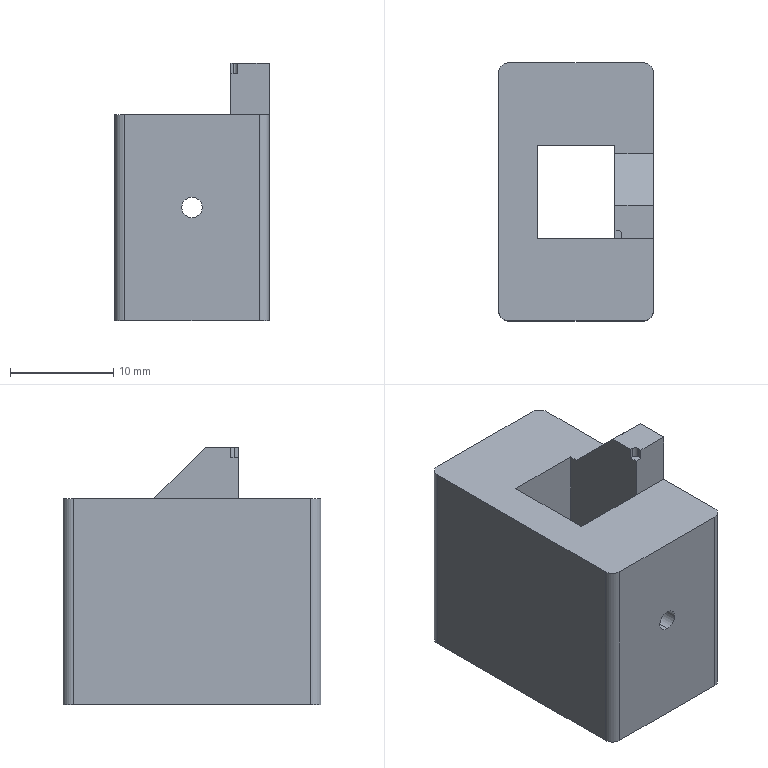Part | STEP file | 03-08 left pre-press cutter plate | 1 solid | 38 faces | box 15 x 25 x 25 mm | volume 5712 mm3 | plane 19 | cylinder 17 | cone 2 | commonest cylinder face diameters 2 x6 3.1 x4 7 x4 4.2 x2 0.7 x1
STEP:
#1=CARTESIAN_POINT('',(0.,-8.5,10.));
#2=VERTEX_POINT('',#1);
#3=CARTESIAN_POINT('',(0.,-8.5,12.));
#4=VERTEX_POINT('',#3);
#5=CARTESIAN_POINT('',(0.,-8.5,11.));
#6=DIRECTION('',(0.,1.,0.));
#7=DIRECTION('',(0.,0.,1.));
#8=AXIS2_PLACEMENT_3D('',#5,#6,#7);
#9=CIRCLE('',#8,1.);
#10=EDGE_CURVE('',#2,#4,#9,.T.);
#11=ORIENTED_EDGE('',*,*,#10,.T.);
#12=CARTESIAN_POINT('',(0.,-12.5,12.));
#13=VERTEX_POINT('',#12);
#14=CARTESIAN_POINT('',(0.,-2.5,12.));
#15=DIRECTION('',(0.,-1.,0.));
#16=VECTOR('',#15,1000.);
#17=LINE('',#14,#16);
#18=EDGE_CURVE('',#4,#13,#17,.T.);
#19=ORIENTED_EDGE('',*,*,#18,.T.);
#20=CARTESIAN_POINT('',(0.,-12.5,10.));
#21=VERTEX_POINT('',#20);
#22=CARTESIAN_POINT('',(0.,-12.5,11.));
#23=DIRECTION('',(0.,-1.,0.));
#24=DIRECTION('',(0.,0.,-1.));
#25=AXIS2_PLACEMENT_3D('',#22,#23,#24);
#26=CIRCLE('',#25,1.);
#27=EDGE_CURVE('',#13,#21,#26,.T.);
#28=ORIENTED_EDGE('',*,*,#27,.T.);
#29=CARTESIAN_POINT('',(0.,-2.5,10.));
#30=DIRECTION('',(0.,-1.,0.));
#31=VECTOR('',#30,1000.);
#32=LINE('',#29,#31);
#33=EDGE_CURVE('',#2,#21,#32,.T.);
#34=ORIENTED_EDGE('',*,*,#33,.F.);
#35=EDGE_LOOP('',(#11,#19,#28,#34));
#36=FACE_OUTER_BOUND('',#35,.T.);
#37=CARTESIAN_POINT('',(0.,-2.5,11.));
#38=DIRECTION('',(0.,-1.,0.));
#39=DIRECTION('',(0.,0.,-1.));
#40=AXIS2_PLACEMENT_3D('',#37,#38,#39);
#41=CYLINDRICAL_SURFACE('',#40,1.);
#42=ADVANCED_FACE('',(#36),#41,.F.);
#43=CARTESIAN_POINT('',(3.5,-8.5,5.));
#44=VERTEX_POINT('',#43);
#45=CARTESIAN_POINT('',(-3.5,-8.5,5.));
#46=VERTEX_POINT('',#45);
#47=CARTESIAN_POINT('',(0.,-8.5,5.));
#48=DIRECTION('',(0.,0.,-1.));
#49=DIRECTION('',(-1.,0.,0.));
#50=AXIS2_PLACEMENT_3D('',#47,#48,#49);
#51=CIRCLE('',#50,3.5);
#52=EDGE_CURVE('',#44,#46,#51,.T.);
#53=ORIENTED_EDGE('',*,*,#52,.F.);
#54=CARTESIAN_POINT('',(3.5,-8.5,0.));
#55=VERTEX_POINT('',#54);
#56=CARTESIAN_POINT('',(3.5,-8.5,5.));
#57=DIRECTION('',(0.,0.,-1.));
#58=VECTOR('',#57,1000.);
#59=LINE('',#56,#58);
#60=EDGE_CURVE('',#44,#55,#59,.T.);
#61=ORIENTED_EDGE('',*,*,#60,.T.);
#62=CARTESIAN_POINT('',(-3.5,-8.5,0.));
#63=VERTEX_POINT('',#62);
#64=CARTESIAN_POINT('',(0.,-8.5,0.));
#65=DIRECTION('',(0.,0.,-1.));
#66=DIRECTION('',(-1.,0.,0.));
#67=AXIS2_PLACEMENT_3D('',#64,#65,#66);
#68=CIRCLE('',#67,3.5);
#69=EDGE_CURVE('',#55,#63,#68,.T.);
#70=ORIENTED_EDGE('',*,*,#69,.T.);
#71=CARTESIAN_POINT('',(-3.5,-8.5,5.));
#72=DIRECTION('',(0.,0.,-1.));
#73=VECTOR('',#72,1000.);
#74=LINE('',#71,#73);
#75=EDGE_CURVE('',#46,#63,#74,.T.);
#76=ORIENTED_EDGE('',*,*,#75,.F.);
#77=EDGE_LOOP('',(#53,#61,#70,#76));
#78=FACE_OUTER_BOUND('',#77,.T.);
#79=CARTESIAN_POINT('',(0.,-8.5,5.));
#80=DIRECTION('',(0.,0.,-1.));
#81=DIRECTION('',(-1.,0.,0.));
#82=AXIS2_PLACEMENT_3D('',#79,#80,#81);
#83=CYLINDRICAL_SURFACE('',#82,3.5);
#84=ADVANCED_FACE('',(#78),#83,.F.);
#85=CARTESIAN_POINT('',(3.5,8.5,5.));
#86=VERTEX_POINT('',#85);
#87=CARTESIAN_POINT('',(-3.5,8.5,5.));
#88=VERTEX_POINT('',#87);
#89=CARTESIAN_POINT('',(0.,8.5,5.));
#90=DIRECTION('',(0.,0.,-1.));
#91=DIRECTION('',(-1.,0.,0.));
#92=AXIS2_PLACEMENT_3D('',#89,#90,#91);
#93=CIRCLE('',#92,3.5);
#94=EDGE_CURVE('',#86,#88,#93,.T.);
#95=ORIENTED_EDGE('',*,*,#94,.F.);
#96=CARTESIAN_POINT('',(3.5,8.5,0.));
#97=VERTEX_POINT('',#96);
#98=CARTESIAN_POINT('',(3.5,8.5,5.));
#99=DIRECTION('',(0.,0.,-1.));
#100=VECTOR('',#99,1000.);
#101=LINE('',#98,#100);
#102=EDGE_CURVE('',#86,#97,#101,.T.);
#103=ORIENTED_EDGE('',*,*,#102,.T.);
#104=CARTESIAN_POINT('',(-3.5,8.5,0.));
#105=VERTEX_POINT('',#104);
#106=CARTESIAN_POINT('',(0.,8.5,0.));
#107=DIRECTION('',(0.,0.,-1.));
#108=DIRECTION('',(-1.,0.,0.));
#109=AXIS2_PLACEMENT_3D('',#106,#107,#108);
#110=CIRCLE('',#109,3.5);
#111=EDGE_CURVE('',#97,#105,#110,.T.);
#112=ORIENTED_EDGE('',*,*,#111,.T.);
#113=CARTESIAN_POINT('',(-3.5,8.5,5.));
#114=DIRECTION('',(0.,0.,-1.));
#115=VECTOR('',#114,1000.);
#116=LINE('',#113,#115);
#117=EDGE_CURVE('',#88,#105,#116,.T.);
#118=ORIENTED_EDGE('',*,*,#117,.F.);
#119=EDGE_LOOP('',(#95,#103,#112,#118));
#120=FACE_OUTER_BOUND('',#119,.T.);
#121=CARTESIAN_POINT('',(0.,8.5,5.));
#122=DIRECTION('',(0.,0.,-1.));
#123=DIRECTION('',(-1.,0.,0.));
#124=AXIS2_PLACEMENT_3D('',#121,#122,#123);
#125=CYLINDRICAL_SURFACE('',#124,3.5);
#126=ADVANCED_FACE('',(#120),#125,.F.);
#127=CARTESIAN_POINT('',(0.,7.5,8.9));
#128=VERTEX_POINT('',#127);
#129=CARTESIAN_POINT('',(0.,7.5,13.1));
#130=VERTEX_POINT('',#129);
#131=CARTESIAN_POINT('',(0.,7.5,11.));
#132=DIRECTION('',(0.,1.,0.));
#133=DIRECTION('',(0.,0.,1.));
#134=AXIS2_PLACEMENT_3D('',#131,#132,#133);
#135=CIRCLE('',#134,2.1);
#136=EDGE_CURVE('',#128,#130,#135,.T.);
#137=ORIENTED_EDGE('',*,*,#136,.F.);
#138=CARTESIAN_POINT('',(0.,12.5,8.9));
#139=VERTEX_POINT('',#138);
#140=CARTESIAN_POINT('',(0.,12.5,8.9));
#141=DIRECTION('',(0.,1.,0.));
#142=VECTOR('',#141,1000.);
#143=LINE('',#140,#142);
#144=EDGE_CURVE('',#128,#139,#143,.T.);
#145=ORIENTED_EDGE('',*,*,#144,.T.);
#146=CARTESIAN_POINT('',(0.,12.5,13.1));
#147=VERTEX_POINT('',#146);
#148=CARTESIAN_POINT('',(0.,12.5,11.));
#149=DIRECTION('',(0.,1.,0.));
#150=DIRECTION('',(0.,0.,1.));
#151=AXIS2_PLACEMENT_3D('',#148,#149,#150);
#152=CIRCLE('',#151,2.1);
#153=EDGE_CURVE('',#139,#147,#152,.T.);
#154=ORIENTED_EDGE('',*,*,#153,.T.);
#155=CARTESIAN_POINT('',(0.,12.5,13.1));
#156=DIRECTION('',(0.,1.,0.));
#157=VECTOR('',#156,1000.);
#158=LINE('',#155,#157);
#159=EDGE_CURVE('',#130,#147,#158,.T.);
#160=ORIENTED_EDGE('',*,*,#159,.F.);
#161=EDGE_LOOP('',(#137,#145,#154,#160));
#162=FACE_OUTER_BOUND('',#161,.T.);
#163=CARTESIAN_POINT('',(0.,12.5,11.));
#164=DIRECTION('',(0.,1.,0.));
#165=DIRECTION('',(0.,0.,1.));
#166=AXIS2_PLACEMENT_3D('',#163,#164,#165);
#167=CYLINDRICAL_SURFACE('',#166,2.1);
#168=ADVANCED_FACE('',(#162),#167,.F.);
#169=CARTESIAN_POINT('',(0.,7.17,9.45));
#170=VERTEX_POINT('',#169);
#171=CARTESIAN_POINT('',(0.,7.17,12.55));
#172=VERTEX_POINT('',#171);
#173=CARTESIAN_POINT('',(0.,7.17,11.));
#174=DIRECTION('',(0.,1.,0.));
#175=DIRECTION('',(0.,0.,1.));
#176=AXIS2_PLACEMENT_3D('',#173,#174,#175);
#177=CIRCLE('',#176,1.55);
#178=EDGE_CURVE('',#170,#172,#177,.T.);
#179=ORIENTED_EDGE('',*,*,#178,.F.);
#180=CARTESIAN_POINT('',(0.,7.5,8.9));
#181=DIRECTION('',(0.,0.515,-0.8572));
#182=VECTOR('',#181,1000.);
#183=LINE('',#180,#182);
#184=EDGE_CURVE('',#170,#128,#183,.T.);
#185=ORIENTED_EDGE('',*,*,#184,.T.);
#186=ORIENTED_EDGE('',*,*,#136,.T.);
#187=CARTESIAN_POINT('',(0.,7.5,13.1));
#188=DIRECTION('',(0.,0.515,0.8572));
#189=VECTOR('',#188,1000.);
#190=LINE('',#187,#189);
#191=EDGE_CURVE('',#172,#130,#190,.T.);
#192=ORIENTED_EDGE('',*,*,#191,.F.);
#193=EDGE_LOOP('',(#179,#185,#186,#192));
#194=FACE_OUTER_BOUND('',#193,.T.);
#195=CARTESIAN_POINT('',(0.,7.5,11.));
#196=DIRECTION('',(0.,1.,0.));
#197=DIRECTION('',(0.,0.,1.));
#198=AXIS2_PLACEMENT_3D('',#195,#196,#197);
#199=CONICAL_SURFACE('',#198,2.1,1.03);
#200=ADVANCED_FACE('',(#194),#199,.F.);
#201=CARTESIAN_POINT('',(0.,4.51,9.45));
#202=VERTEX_POINT('',#201);
#203=CARTESIAN_POINT('',(0.,4.51,12.55));
#204=VERTEX_POINT('',#203);
#205=CARTESIAN_POINT('',(0.,4.51,11.));
#206=DIRECTION('',(0.,1.,0.));
#207=DIRECTION('',(0.,0.,1.));
#208=AXIS2_PLACEMENT_3D('',#205,#206,#207);
#209=CIRCLE('',#208,1.55);
#210=EDGE_CURVE('',#202,#204,#209,.T.);
#211=ORIENTED_EDGE('',*,*,#210,.F.);
#212=CARTESIAN_POINT('',(0.,-8.5,9.45));
#213=DIRECTION('',(0.,1.,0.));
#214=VECTOR('',#213,1000.);
#215=LINE('',#212,#214);
#216=EDGE_CURVE('',#202,#170,#215,.T.);
#217=ORIENTED_EDGE('',*,*,#216,.T.);
#218=ORIENTED_EDGE('',*,*,#178,.T.);
#219=CARTESIAN_POINT('',(0.,-8.5,12.55));
#220=DIRECTION('',(0.,1.,0.));
#221=VECTOR('',#220,1000.);
#222=LINE('',#219,#221);
#223=EDGE_CURVE('',#204,#172,#222,.T.);
#224=ORIENTED_EDGE('',*,*,#223,.F.);
#225=EDGE_LOOP('',(#211,#217,#218,#224));
#226=FACE_OUTER_BOUND('',#225,.T.);
#227=CARTESIAN_POINT('',(0.,-8.5,11.));
#228=DIRECTION('',(0.,1.,0.));
#229=DIRECTION('',(0.,0.,1.));
#230=AXIS2_PLACEMENT_3D('',#227,#228,#229);
#231=CYLINDRICAL_SURFACE('',#230,1.55);
#232=ADVANCED_FACE('',(#226),#231,.F.);
#233=CARTESIAN_POINT('',(0.,-8.5,9.45));
#234=VERTEX_POINT('',#233);
#235=CARTESIAN_POINT('',(0.,-8.5,12.55));
#236=VERTEX_POINT('',#235);
#237=CARTESIAN_POINT('',(0.,-8.5,11.));
#238=DIRECTION('',(0.,1.,0.));
#239=DIRECTION('',(0.,0.,1.));
#240=AXIS2_PLACEMENT_3D('',#237,#238,#239);
#241=CIRCLE('',#240,1.55);
#242=EDGE_CURVE('',#234,#236,#241,.T.);
#243=ORIENTED_EDGE('',*,*,#242,.F.);
#244=CARTESIAN_POINT('',(0.,-4.51,9.45));
#245=VERTEX_POINT('',#244);
#246=CARTESIAN_POINT('',(0.,-8.5,9.45));
#247=DIRECTION('',(0.,1.,0.));
#248=VECTOR('',#247,1000.);
#249=LINE('',#246,#248);
#250=EDGE_CURVE('',#234,#245,#249,.T.);
#251=ORIENTED_EDGE('',*,*,#250,.T.);
#252=CARTESIAN_POINT('',(0.,-4.51,12.55));
#253=VERTEX_POINT('',#252);
#254=CARTESIAN_POINT('',(0.,-4.51,11.));
#255=DIRECTION('',(0.,-1.,0.));
#256=DIRECTION('',(0.,0.,-1.));
#257=AXIS2_PLACEMENT_3D('',#254,#255,#256);
#258=CIRCLE('',#257,1.55);
#259=EDGE_CURVE('',#253,#245,#258,.T.);
#260=ORIENTED_EDGE('',*,*,#259,.F.);
#261=CARTESIAN_POINT('',(0.,-8.5,12.55));
#262=DIRECTION('',(0.,1.,0.));
#263=VECTOR('',#262,1000.);
#264=LINE('',#261,#263);
#265=EDGE_CURVE('',#236,#253,#264,.T.);
#266=ORIENTED_EDGE('',*,*,#265,.F.);
#267=EDGE_LOOP('',(#243,#251,#260,#266));
#268=FACE_OUTER_BOUND('',#267,.T.);
#269=CARTESIAN_POINT('',(0.,-8.5,11.));
#270=DIRECTION('',(0.,1.,0.));
#271=DIRECTION('',(0.,0.,1.));
#272=AXIS2_PLACEMENT_3D('',#269,#270,#271);
#273=CYLINDRICAL_SURFACE('',#272,1.55);
#274=ADVANCED_FACE('',(#268),#273,.F.);
#275=CARTESIAN_POINT('',(0.,12.5,11.));
#276=DIRECTION('',(0.,1.,0.));
#277=DIRECTION('',(0.,0.,1.));
#278=AXIS2_PLACEMENT_3D('',#275,#276,#277);
#279=CIRCLE('',#278,2.1);
#280=EDGE_CURVE('',#147,#139,#279,.T.);
#281=ORIENTED_EDGE('',*,*,#280,.F.);
#282=ORIENTED_EDGE('',*,*,#153,.F.);
#283=EDGE_LOOP('',(#281,#282));
#284=FACE_BOUND('',#283,.T.);
#285=CARTESIAN_POINT('',(6.5,12.5,0.));
#286=VERTEX_POINT('',#285);
#287=CARTESIAN_POINT('',(-6.5,12.5,0.));
#288=VERTEX_POINT('',#287);
#289=CARTESIAN_POINT('',(-7.5,12.5,0.));
#290=DIRECTION('',(-1.,0.,0.));
#291=VECTOR('',#290,1000.);
#292=LINE('',#289,#291);
#293=EDGE_CURVE('',#286,#288,#292,.T.);
#294=ORIENTED_EDGE('',*,*,#293,.T.);
#295=CARTESIAN_POINT('',(-6.5,12.5,20.));
#296=VERTEX_POINT('',#295);
#297=CARTESIAN_POINT('',(-6.5,12.5,25.));
#298=DIRECTION('',(0.,0.,1.));
#299=VECTOR('',#298,1000.);
#300=LINE('',#297,#299);
#301=EDGE_CURVE('',#288,#296,#300,.T.);
#302=ORIENTED_EDGE('',*,*,#301,.T.);
#303=CARTESIAN_POINT('',(6.5,12.5,20.));
#304=VERTEX_POINT('',#303);
#305=CARTESIAN_POINT('',(-7.5,12.5,20.));
#306=DIRECTION('',(-1.,0.,0.));
#307=VECTOR('',#306,1000.);
#308=LINE('',#305,#307);
#309=EDGE_CURVE('',#304,#296,#308,.T.);
#310=ORIENTED_EDGE('',*,*,#309,.F.);
#311=CARTESIAN_POINT('',(6.5,12.5,25.));
#312=DIRECTION('',(0.,0.,-1.));
#313=VECTOR('',#312,1000.);
#314=LINE('',#311,#313);
#315=EDGE_CURVE('',#304,#286,#314,.T.);
#316=ORIENTED_EDGE('',*,*,#315,.T.);
#317=EDGE_LOOP('',(#294,#302,#310,#316));
#318=FACE_OUTER_BOUND('',#317,.T.);
#319=CARTESIAN_POINT('',(-7.5,12.5,25.));
#320=DIRECTION('',(0.,-1.,0.));
#321=DIRECTION('',(0.,0.,-1.));
#322=AXIS2_PLACEMENT_3D('',#319,#320,#321);
#323=PLANE('',#322);
#324=ADVANCED_FACE('',(#284,#318),#323,.F.);
#325=CARTESIAN_POINT('',(-7.5,11.5,20.));
#326=VERTEX_POINT('',#325);
#327=CARTESIAN_POINT('',(-7.5,-11.5,20.));
#328=VERTEX_POINT('',#327);
#329=CARTESIAN_POINT('',(-7.5,12.5,20.));
#330=DIRECTION('',(0.,-1.,0.));
#331=VECTOR('',#330,1000.);
#332=LINE('',#329,#331);
#333=EDGE_CURVE('',#326,#328,#332,.T.);
#334=ORIENTED_EDGE('',*,*,#333,.F.);
#335=CARTESIAN_POINT('',(-7.5,11.5,0.));
#336=VERTEX_POINT('',#335);
#337=CARTESIAN_POINT('',(-7.5,11.5,25.));
#338=DIRECTION('',(0.,0.,-1.));
#339=VECTOR('',#338,1000.);
#340=LINE('',#337,#339);
#341=EDGE_CURVE('',#326,#336,#340,.T.);
#342=ORIENTED_EDGE('',*,*,#341,.T.);
#343=CARTESIAN_POINT('',(-7.5,-11.5,0.));
#344=VERTEX_POINT('',#343);
#345=CARTESIAN_POINT('',(-7.5,12.5,0.));
#346=DIRECTION('',(0.,-1.,0.));
#347=VECTOR('',#346,1000.);
#348=LINE('',#345,#347);
#349=EDGE_CURVE('',#336,#344,#348,.T.);
#350=ORIENTED_EDGE('',*,*,#349,.T.);
#351=CARTESIAN_POINT('',(-7.5,-11.5,25.));
#352=DIRECTION('',(0.,0.,1.));
#353=VECTOR('',#352,1000.);
#354=LINE('',#351,#353);
#355=EDGE_CURVE('',#344,#328,#354,.T.);
#356=ORIENTED_EDGE('',*,*,#355,.T.);
#357=EDGE_LOOP('',(#334,#342,#350,#356));
#358=FACE_OUTER_BOUND('',#357,.T.);
#359=CARTESIAN_POINT('',(-7.5,12.5,25.));
#360=DIRECTION('',(1.,0.,0.));
#361=DIRECTION('',(0.,1.,0.));
#362=AXIS2_PLACEMENT_3D('',#359,#360,#361);
#363=PLANE('',#362);
#364=ADVANCED_FACE('',(#358),#363,.F.);
#365=CARTESIAN_POINT('',(0.,-12.5,11.));
#366=DIRECTION('',(0.,-1.,0.));
#367=DIRECTION('',(0.,0.,-1.));
#368=AXIS2_PLACEMENT_3D('',#365,#366,#367);
#369=CIRCLE('',#368,1.);
#370=EDGE_CURVE('',#21,#13,#369,.T.);
#371=ORIENTED_EDGE('',*,*,#370,.F.);
#372=ORIENTED_EDGE('',*,*,#27,.F.);
#373=EDGE_LOOP('',(#371,#372));
#374=FACE_BOUND('',#373,.T.);
#375=CARTESIAN_POINT('',(-6.5,-12.5,20.));
#376=VERTEX_POINT('',#375);
#377=CARTESIAN_POINT('',(6.5,-12.5,20.));
#378=VERTEX_POINT('',#377);
#379=CARTESIAN_POINT('',(-7.5,-12.5,20.));
#380=DIRECTION('',(1.,0.,0.));
#381=VECTOR('',#380,1000.);
#382=LINE('',#379,#381);
#383=EDGE_CURVE('',#376,#378,#382,.T.);
#384=ORIENTED_EDGE('',*,*,#383,.F.);
#385=CARTESIAN_POINT('',(-6.5,-12.5,0.));
#386=VERTEX_POINT('',#385);
#387=CARTESIAN_POINT('',(-6.5,-12.5,25.));
#388=DIRECTION('',(0.,0.,-1.));
#389=VECTOR('',#388,1000.);
#390=LINE('',#387,#389);
#391=EDGE_CURVE('',#376,#386,#390,.T.);
#392=ORIENTED_EDGE('',*,*,#391,.T.);
#393=CARTESIAN_POINT('',(6.5,-12.5,0.));
#394=VERTEX_POINT('',#393);
#395=CARTESIAN_POINT('',(-7.5,-12.5,0.));
#396=DIRECTION('',(1.,0.,0.));
#397=VECTOR('',#396,1000.);
#398=LINE('',#395,#397);
#399=EDGE_CURVE('',#386,#394,#398,.T.);
#400=ORIENTED_EDGE('',*,*,#399,.T.);
#401=CARTESIAN_POINT('',(6.5,-12.5,25.));
#402=DIRECTION('',(0.,0.,1.));
#403=VECTOR('',#402,1000.);
#404=LINE('',#401,#403);
#405=EDGE_CURVE('',#394,#378,#404,.T.);
#406=ORIENTED_EDGE('',*,*,#405,.T.);
#407=EDGE_LOOP('',(#384,#392,#400,#406));
#408=FACE_OUTER_BOUND('',#407,.T.);
#409=CARTESIAN_POINT('',(-7.5,-12.5,25.));
#410=DIRECTION('',(0.,1.,0.));
#411=DIRECTION('',(0.,0.,1.));
#412=AXIS2_PLACEMENT_3D('',#409,#410,#411);
#413=PLANE('',#412);
#414=ADVANCED_FACE('',(#374,#408),#413,.F.);
#415=CARTESIAN_POINT('',(-3.76,-4.51,20.));
#416=VERTEX_POINT('',#415);
#417=CARTESIAN_POINT('',(-3.76,4.51,20.));
#418=VERTEX_POINT('',#417);
#419=CARTESIAN_POINT('',(-3.76,4.51,20.));
#420=DIRECTION('',(0.,1.,0.));
#421=VECTOR('',#420,1000.);
#422=LINE('',#419,#421);
#423=EDGE_CURVE('',#416,#418,#422,.T.);
#424=ORIENTED_EDGE('',*,*,#423,.F.);
#425=CARTESIAN_POINT('',(-3.76,-4.51,0.));
#426=VERTEX_POINT('',#425);
#427=CARTESIAN_POINT('',(-3.76,-4.51,0.));
#428=DIRECTION('',(0.,0.,1.));
#429=VECTOR('',#428,1000.);
#430=LINE('',#427,#429);
#431=EDGE_CURVE('',#426,#416,#430,.T.);
#432=ORIENTED_EDGE('',*,*,#431,.F.);
#433=CARTESIAN_POINT('',(-3.76,4.51,0.));
#434=VERTEX_POINT('',#433);
#435=CARTESIAN_POINT('',(-3.76,4.51,0.));
#436=DIRECTION('',(0.,-1.,0.));
#437=VECTOR('',#436,1000.);
#438=LINE('',#435,#437);
#439=EDGE_CURVE('',#434,#426,#438,.T.);
#440=ORIENTED_EDGE('',*,*,#439,.F.);
#441=CARTESIAN_POINT('',(-3.76,4.51,0.));
#442=DIRECTION('',(0.,0.,1.));
#443=VECTOR('',#442,1000.);
#444=LINE('',#441,#443);
#445=EDGE_CURVE('',#434,#418,#444,.T.);
#446=ORIENTED_EDGE('',*,*,#445,.T.);
#447=EDGE_LOOP('',(#424,#432,#440,#446));
#448=FACE_OUTER_BOUND('',#447,.T.);
#449=CARTESIAN_POINT('',(-3.76,4.51,0.));
#450=DIRECTION('',(-1.,0.,0.));
#451=DIRECTION('',(0.,-1.,0.));
#452=AXIS2_PLACEMENT_3D('',#449,#450,#451);
#453=PLANE('',#452);
#454=ADVANCED_FACE('',(#448),#453,.F.);
#455=CARTESIAN_POINT('',(0.,4.51,11.));
#456=DIRECTION('',(0.,1.,0.));
#457=DIRECTION('',(0.,0.,1.));
#458=AXIS2_PLACEMENT_3D('',#455,#456,#457);
#459=CIRCLE('',#458,1.55);
#460=EDGE_CURVE('',#204,#202,#459,.T.);
#461=ORIENTED_EDGE('',*,*,#460,.T.);
#462=ORIENTED_EDGE('',*,*,#210,.T.);
#463=EDGE_LOOP('',(#461,#462));
#464=FACE_BOUND('',#463,.T.);
#465=CARTESIAN_POINT('',(3.76,4.51,20.));
#466=VERTEX_POINT('',#465);
#467=CARTESIAN_POINT('',(-3.76,4.51,20.));
#468=DIRECTION('',(1.,0.,0.));
#469=VECTOR('',#468,1000.);
#470=LINE('',#467,#469);
#471=EDGE_CURVE('',#418,#466,#470,.T.);
#472=ORIENTED_EDGE('',*,*,#471,.F.);
#473=ORIENTED_EDGE('',*,*,#445,.F.);
#474=CARTESIAN_POINT('',(3.76,4.51,0.));
#475=VERTEX_POINT('',#474);
#476=CARTESIAN_POINT('',(-3.76,4.51,0.));
#477=DIRECTION('',(-1.,0.,0.));
#478=VECTOR('',#477,1000.);
#479=LINE('',#476,#478);
#480=EDGE_CURVE('',#475,#434,#479,.T.);
#481=ORIENTED_EDGE('',*,*,#480,.F.);
#482=CARTESIAN_POINT('',(3.76,4.51,0.));
#483=DIRECTION('',(0.,0.,1.));
#484=VECTOR('',#483,1000.);
#485=LINE('',#482,#484);
#486=EDGE_CURVE('',#475,#466,#485,.T.);
#487=ORIENTED_EDGE('',*,*,#486,.T.);
#488=EDGE_LOOP('',(#472,#473,#481,#487));
#489=FACE_OUTER_BOUND('',#488,.T.);
#490=CARTESIAN_POINT('',(-3.76,4.51,0.));
#491=DIRECTION('',(0.,1.,0.));
#492=DIRECTION('',(0.,0.,1.));
#493=AXIS2_PLACEMENT_3D('',#490,#491,#492);
#494=PLANE('',#493);
#495=ADVANCED_FACE('',(#464,#489),#494,.F.);
#496=ORIENTED_EDGE('',*,*,#259,.T.);
#497=CARTESIAN_POINT('',(0.,-4.51,11.));
#498=DIRECTION('',(0.,-1.,0.));
#499=DIRECTION('',(0.,0.,-1.));
#500=AXIS2_PLACEMENT_3D('',#497,#498,#499);
#501=CIRCLE('',#500,1.55);
#502=EDGE_CURVE('',#245,#253,#501,.T.);
#503=ORIENTED_EDGE('',*,*,#502,.T.);
#504=EDGE_LOOP('',(#496,#503));
#505=FACE_BOUND('',#504,.T.);
#506=CARTESIAN_POINT('',(3.76,-4.51,20.));
#507=VERTEX_POINT('',#506);
#508=CARTESIAN_POINT('',(-3.76,-4.51,20.));
#509=DIRECTION('',(-1.,0.,0.));
#510=VECTOR('',#509,1000.);
#511=LINE('',#508,#510);
#512=EDGE_CURVE('',#507,#416,#511,.T.);
#513=ORIENTED_EDGE('',*,*,#512,.F.);
#514=CARTESIAN_POINT('',(3.76,-4.51,0.));
#515=VERTEX_POINT('',#514);
#516=CARTESIAN_POINT('',(3.76,-4.51,0.));
#517=DIRECTION('',(0.,0.,1.));
#518=VECTOR('',#517,1000.);
#519=LINE('',#516,#518);
#520=EDGE_CURVE('',#515,#507,#519,.T.);
#521=ORIENTED_EDGE('',*,*,#520,.F.);
#522=CARTESIAN_POINT('',(-3.76,-4.51,0.));
#523=DIRECTION('',(1.,0.,0.));
#524=VECTOR('',#523,1000.);
#525=LINE('',#522,#524);
#526=EDGE_CURVE('',#426,#515,#525,.T.);
#527=ORIENTED_EDGE('',*,*,#526,.F.);
#528=ORIENTED_EDGE('',*,*,#431,.T.);
#529=EDGE_LOOP('',(#513,#521,#527,#528));
#530=FACE_OUTER_BOUND('',#529,.T.);
#531=CARTESIAN_POINT('',(-3.76,-4.51,0.));
#532=DIRECTION('',(0.,-1.,0.));
#533=DIRECTION('',(0.,0.,-1.));
#534=AXIS2_PLACEMENT_3D('',#531,#532,#533);
#535=PLANE('',#534);
#536=ADVANCED_FACE('',(#505,#530),#535,.F.);
#537=CARTESIAN_POINT('',(7.5,-11.5,20.));
#538=VERTEX_POINT('',#537);
#539=CARTESIAN_POINT('',(7.5,-4.5,20.));
#540=VERTEX_POINT('',#539);
#541=CARTESIAN_POINT('',(7.5,12.5,20.));
#542=DIRECTION('',(0.,1.,0.));
#543=VECTOR('',#542,1000.);
#544=LINE('',#541,#543);
#545=EDGE_CURVE('',#538,#540,#544,.T.);
#546=ORIENTED_EDGE('',*,*,#545,.F.);
#547=CARTESIAN_POINT('',(7.5,-11.5,0.));
#548=VERTEX_POINT('',#547);
#549=CARTESIAN_POINT('',(7.5,-11.5,25.));
#550=DIRECTION('',(0.,0.,-1.));
#551=VECTOR('',#550,1000.);
#552=LINE('',#549,#551);
#553=EDGE_CURVE('',#538,#548,#552,.T.);
#554=ORIENTED_EDGE('',*,*,#553,.T.);
#555=CARTESIAN_POINT('',(7.5,11.5,0.));
#556=VERTEX_POINT('',#555);
#557=CARTESIAN_POINT('',(7.5,12.5,0.));
#558=DIRECTION('',(0.,1.,0.));
#559=VECTOR('',#558,1000.);
#560=LINE('',#557,#559);
#561=EDGE_CURVE('',#548,#556,#560,.T.);
#562=ORIENTED_EDGE('',*,*,#561,.T.);
#563=CARTESIAN_POINT('',(7.5,11.5,20.));
#564=VERTEX_POINT('',#563);
#565=CARTESIAN_POINT('',(7.5,11.5,25.));
#566=DIRECTION('',(0.,0.,1.));
#567=VECTOR('',#566,1000.);
#568=LINE('',#565,#567);
#569=EDGE_CURVE('',#556,#564,#568,.T.);
#570=ORIENTED_EDGE('',*,*,#569,.T.);
#571=CARTESIAN_POINT('',(7.5,3.7,20.));
#572=VERTEX_POINT('',#571);
#573=CARTESIAN_POINT('',(7.5,12.5,20.));
#574=DIRECTION('',(0.,1.,0.));
#575=VECTOR('',#574,1000.);
#576=LINE('',#573,#575);
#577=EDGE_CURVE('',#572,#564,#576,.T.);
#578=ORIENTED_EDGE('',*,*,#577,.F.);
#579=CARTESIAN_POINT('',(7.5,-1.3,25.));
#580=VERTEX_POINT('',#579);
#581=CARTESIAN_POINT('',(7.5,-1.3,25.));
#582=DIRECTION('',(0.,-0.7071,0.7071));
#583=VECTOR('',#582,1000.);
#584=LINE('',#581,#583);
#585=EDGE_CURVE('',#572,#580,#584,.T.);
#586=ORIENTED_EDGE('',*,*,#585,.T.);
#587=CARTESIAN_POINT('',(7.5,-4.5,25.));
#588=VERTEX_POINT('',#587);
#589=CARTESIAN_POINT('',(7.5,12.5,25.));
#590=DIRECTION('',(0.,1.,0.));
#591=VECTOR('',#590,1000.);
#592=LINE('',#589,#591);
#593=EDGE_CURVE('',#588,#580,#592,.T.);
#594=ORIENTED_EDGE('',*,*,#593,.F.);
#595=CARTESIAN_POINT('',(7.5,-4.5,25.));
#596=DIRECTION('',(0.,0.,-1.));
#597=VECTOR('',#596,1000.);
#598=LINE('',#595,#597);
#599=EDGE_CURVE('',#588,#540,#598,.T.);
#600=ORIENTED_EDGE('',*,*,#599,.T.);
#601=EDGE_LOOP('',(#546,#554,#562,#570,#578,#586,#594,#600));
#602=FACE_OUTER_BOUND('',#601,.T.);
#603=CARTESIAN_POINT('',(7.5,12.5,25.));
#604=DIRECTION('',(-1.,0.,0.));
#605=DIRECTION('',(0.,-1.,0.));
#606=AXIS2_PLACEMENT_3D('',#603,#604,#605);
#607=PLANE('',#606);
#608=ADVANCED_FACE('',(#602),#607,.F.);
#609=CARTESIAN_POINT('',(4.4,-4.5,25.));
#610=VERTEX_POINT('',#609);
#611=CARTESIAN_POINT('',(4.4,-4.1,25.));
#612=VERTEX_POINT('',#611);
#613=CARTESIAN_POINT('',(4.4,-4.1,25.));
#614=DIRECTION('',(0.,1.,0.));
#615=VECTOR('',#614,1000.);
#616=LINE('',#613,#615);
#617=EDGE_CURVE('',#610,#612,#616,.T.);
#618=ORIENTED_EDGE('',*,*,#617,.F.);
#619=CARTESIAN_POINT('',(-3.75,-4.5,25.));
#620=DIRECTION('',(-1.,0.,0.));
#621=VECTOR('',#620,1000.);
#622=LINE('',#619,#621);
#623=EDGE_CURVE('',#588,#610,#622,.T.);
#624=ORIENTED_EDGE('',*,*,#623,.F.);
#625=ORIENTED_EDGE('',*,*,#593,.T.);
#626=CARTESIAN_POINT('',(3.76,-1.3,25.));
#627=VERTEX_POINT('',#626);
#628=CARTESIAN_POINT('',(-3.75,-1.3,25.));
#629=DIRECTION('',(1.,0.,0.));
#630=VECTOR('',#629,1000.);
#631=LINE('',#628,#630);
#632=EDGE_CURVE('',#627,#580,#631,.T.);
#633=ORIENTED_EDGE('',*,*,#632,.F.);
#634=CARTESIAN_POINT('',(3.76,-3.75,25.));
#635=VERTEX_POINT('',#634);
#636=CARTESIAN_POINT('',(3.76,4.51,25.));
#637=DIRECTION('',(0.,1.,0.));
#638=VECTOR('',#637,1000.);
#639=LINE('',#636,#638);
#640=EDGE_CURVE('',#635,#627,#639,.T.);
#641=ORIENTED_EDGE('',*,*,#640,.F.);
#642=CARTESIAN_POINT('',(4.05,-3.75,25.));
#643=VERTEX_POINT('',#642);
#644=CARTESIAN_POINT('',(4.05,-3.75,25.));
#645=DIRECTION('',(-1.,0.,0.));
#646=VECTOR('',#645,1000.);
#647=LINE('',#644,#646);
#648=EDGE_CURVE('',#643,#635,#647,.T.);
#649=ORIENTED_EDGE('',*,*,#648,.F.);
#650=CARTESIAN_POINT('',(4.05,-4.1,25.));
#651=DIRECTION('',(0.,0.,1.));
#652=DIRECTION('',(1.,0.,0.));
#653=AXIS2_PLACEMENT_3D('',#650,#651,#652);
#654=CIRCLE('',#653,0.35);
#655=EDGE_CURVE('',#612,#643,#654,.T.);
#656=ORIENTED_EDGE('',*,*,#655,.F.);
#657=EDGE_LOOP('',(#618,#624,#625,#633,#641,#649,#656));
#658=FACE_OUTER_BOUND('',#657,.T.);
#659=CARTESIAN_POINT('',(7.5,-12.5,25.));
#660=DIRECTION('',(0.,0.,1.));
#661=DIRECTION('',(1.,0.,0.));
#662=AXIS2_PLACEMENT_3D('',#659,#660,#661);
#663=PLANE('',#662);
#664=ADVANCED_FACE('',(#658),#663,.T.);
#665=CARTESIAN_POINT('',(0.,-8.5,0.));
#666=DIRECTION('',(0.,0.,-1.));
#667=DIRECTION('',(-1.,0.,0.));
#668=AXIS2_PLACEMENT_3D('',#665,#666,#667);
#669=CIRCLE('',#668,3.5);
#670=EDGE_CURVE('',#63,#55,#669,.T.);
#671=ORIENTED_EDGE('',*,*,#670,.F.);
#672=ORIENTED_EDGE('',*,*,#69,.F.);
#673=EDGE_LOOP('',(#671,#672));
#674=FACE_BOUND('',#673,.T.);
#675=CARTESIAN_POINT('',(0.,8.5,0.));
#676=DIRECTION('',(0.,0.,-1.));
#677=DIRECTION('',(-1.,0.,0.));
#678=AXIS2_PLACEMENT_3D('',#675,#676,#677);
#679=CIRCLE('',#678,3.5);
#680=EDGE_CURVE('',#105,#97,#679,.T.);
#681=ORIENTED_EDGE('',*,*,#680,.F.);
#682=ORIENTED_EDGE('',*,*,#111,.F.);
#683=EDGE_LOOP('',(#681,#682));
#684=FACE_BOUND('',#683,.T.);
#685=ORIENTED_EDGE('',*,*,#480,.T.);
#686=ORIENTED_EDGE('',*,*,#439,.T.);
#687=ORIENTED_EDGE('',*,*,#526,.T.);
#688=CARTESIAN_POINT('',(3.76,4.51,0.));
#689=DIRECTION('',(0.,1.,0.));
#690=VECTOR('',#689,1000.);
#691=LINE('',#688,#690);
#692=EDGE_CURVE('',#515,#475,#691,.T.);
#693=ORIENTED_EDGE('',*,*,#692,.T.);
#694=EDGE_LOOP('',(#685,#686,#687,#693));
#695=FACE_BOUND('',#694,.T.);
#696=ORIENTED_EDGE('',*,*,#349,.F.);
#697=CARTESIAN_POINT('',(-6.5,11.5,0.));
#698=DIRECTION('',(0.,0.,-1.));
#699=DIRECTION('',(1.,0.,0.));
#700=AXIS2_PLACEMENT_3D('',#697,#698,#699);
#701=CIRCLE('',#700,1.);
#702=EDGE_CURVE('',#336,#288,#701,.T.);
#703=ORIENTED_EDGE('',*,*,#702,.T.);
#704=ORIENTED_EDGE('',*,*,#293,.F.);
#705=CARTESIAN_POINT('',(6.5,11.5,0.));
#706=DIRECTION('',(0.,0.,-1.));
#707=DIRECTION('',(1.,0.,0.));
#708=AXIS2_PLACEMENT_3D('',#705,#706,#707);
#709=CIRCLE('',#708,1.);
#710=EDGE_CURVE('',#286,#556,#709,.T.);
#711=ORIENTED_EDGE('',*,*,#710,.T.);
#712=ORIENTED_EDGE('',*,*,#561,.F.);
#713=CARTESIAN_POINT('',(6.5,-11.5,0.));
#714=DIRECTION('',(0.,0.,-1.));
#715=DIRECTION('',(1.,0.,0.));
#716=AXIS2_PLACEMENT_3D('',#713,#714,#715);
#717=CIRCLE('',#716,1.);
#718=EDGE_CURVE('',#548,#394,#717,.T.);
#719=ORIENTED_EDGE('',*,*,#718,.T.);
#720=ORIENTED_EDGE('',*,*,#399,.F.);
#721=CARTESIAN_POINT('',(-6.5,-11.5,0.));
#722=DIRECTION('',(0.,0.,-1.));
#723=DIRECTION('',(1.,0.,0.));
#724=AXIS2_PLACEMENT_3D('',#721,#722,#723);
#725=CIRCLE('',#724,1.);
#726=EDGE_CURVE('',#386,#344,#725,.T.);
#727=ORIENTED_EDGE('',*,*,#726,.T.);
#728=EDGE_LOOP('',(#696,#703,#704,#711,#712,#719,#720,#727));
#729=FACE_OUTER_BOUND('',#728,.T.);
#730=CARTESIAN_POINT('',(7.5,-12.5,0.));
#731=DIRECTION('',(0.,0.,1.));
#732=DIRECTION('',(1.,0.,0.));
#733=AXIS2_PLACEMENT_3D('',#730,#731,#732);
#734=PLANE('',#733);
#735=ADVANCED_FACE('',(#674,#684,#695,#729),#734,.F.);
#736=CARTESIAN_POINT('',(3.76,-3.75,24.));
#737=VERTEX_POINT('',#736);
#738=CARTESIAN_POINT('',(3.76,-4.5,24.));
#739=VERTEX_POINT('',#738);
#740=CARTESIAN_POINT('',(3.76,4.51,24.));
#741=DIRECTION('',(0.,-1.,0.));
#742=VECTOR('',#741,1000.);
#743=LINE('',#740,#742);
#744=EDGE_CURVE('',#737,#739,#743,.T.);
#745=ORIENTED_EDGE('',*,*,#744,.F.);
#746=CARTESIAN_POINT('',(3.76,-3.75,0.));
#747=DIRECTION('',(0.,0.,1.));
#748=VECTOR('',#747,1000.);
#749=LINE('',#746,#748);
#750=EDGE_CURVE('',#737,#635,#749,.T.);
#751=ORIENTED_EDGE('',*,*,#750,.T.);
#752=ORIENTED_EDGE('',*,*,#640,.T.);
#753=CARTESIAN_POINT('',(3.76,3.7,20.));
#754=VERTEX_POINT('',#753);
#755=CARTESIAN_POINT('',(3.76,-1.3,25.));
#756=DIRECTION('',(0.,0.7071,-0.7071));
#757=VECTOR('',#756,1000.);
#758=LINE('',#755,#757);
#759=EDGE_CURVE('',#627,#754,#758,.T.);
#760=ORIENTED_EDGE('',*,*,#759,.T.);
#761=CARTESIAN_POINT('',(3.76,4.51,20.));
#762=DIRECTION('',(0.,-1.,0.));
#763=VECTOR('',#762,1000.);
#764=LINE('',#761,#763);
#765=EDGE_CURVE('',#466,#754,#764,.T.);
#766=ORIENTED_EDGE('',*,*,#765,.F.);
#767=ORIENTED_EDGE('',*,*,#486,.F.);
#768=ORIENTED_EDGE('',*,*,#692,.F.);
#769=ORIENTED_EDGE('',*,*,#520,.T.);
#770=CARTESIAN_POINT('',(3.76,-4.5,20.));
#771=VERTEX_POINT('',#770);
#772=CARTESIAN_POINT('',(3.76,4.51,20.));
#773=DIRECTION('',(0.,-1.,0.));
#774=VECTOR('',#773,1000.);
#775=LINE('',#772,#774);
#776=EDGE_CURVE('',#771,#507,#775,.T.);
#777=ORIENTED_EDGE('',*,*,#776,.F.);
#778=CARTESIAN_POINT('',(3.76,-4.5,0.));
#779=DIRECTION('',(0.,0.,1.));
#780=VECTOR('',#779,1000.);
#781=LINE('',#778,#780);
#782=EDGE_CURVE('',#771,#739,#781,.T.);
#783=ORIENTED_EDGE('',*,*,#782,.T.);
#784=EDGE_LOOP('',(#745,#751,#752,#760,#766,#767,#768,#769,#777,#783));
#785=FACE_OUTER_BOUND('',#784,.T.);
#786=CARTESIAN_POINT('',(3.76,4.51,0.));
#787=DIRECTION('',(1.,0.,0.));
#788=DIRECTION('',(0.,1.,0.));
#789=AXIS2_PLACEMENT_3D('',#786,#787,#788);
#790=PLANE('',#789);
#791=ADVANCED_FACE('',(#785),#790,.F.);
#792=ORIENTED_EDGE('',*,*,#623,.T.);
#793=CARTESIAN_POINT('',(4.4,-4.5,24.));
#794=VERTEX_POINT('',#793);
#795=CARTESIAN_POINT('',(4.4,-4.5,20.));
#796=DIRECTION('',(0.,0.,-1.));
#797=VECTOR('',#796,1000.);
#798=LINE('',#795,#797);
#799=EDGE_CURVE('',#610,#794,#798,.T.);
#800=ORIENTED_EDGE('',*,*,#799,.T.);
#801=CARTESIAN_POINT('',(-3.75,-4.5,24.));
#802=DIRECTION('',(1.,0.,0.));
#803=VECTOR('',#802,1000.);
#804=LINE('',#801,#803);
#805=EDGE_CURVE('',#739,#794,#804,.T.);
#806=ORIENTED_EDGE('',*,*,#805,.F.);
#807=ORIENTED_EDGE('',*,*,#782,.F.);
#808=CARTESIAN_POINT('',(-3.75,-4.5,20.));
#809=DIRECTION('',(-1.,0.,0.));
#810=VECTOR('',#809,1000.);
#811=LINE('',#808,#810);
#812=EDGE_CURVE('',#540,#771,#811,.T.);
#813=ORIENTED_EDGE('',*,*,#812,.F.);
#814=ORIENTED_EDGE('',*,*,#599,.F.);
#815=EDGE_LOOP('',(#792,#800,#806,#807,#813,#814));
#816=FACE_OUTER_BOUND('',#815,.T.);
#817=CARTESIAN_POINT('',(-3.75,-4.5,20.));
#818=DIRECTION('',(0.,1.,0.));
#819=DIRECTION('',(0.,0.,1.));
#820=AXIS2_PLACEMENT_3D('',#817,#818,#819);
#821=PLANE('',#820);
#822=ADVANCED_FACE('',(#816),#821,.F.);
#823=ORIENTED_EDGE('',*,*,#309,.T.);
#824=CARTESIAN_POINT('',(-6.5,11.5,20.));
#825=DIRECTION('',(0.,0.,1.));
#826=DIRECTION('',(1.,0.,0.));
#827=AXIS2_PLACEMENT_3D('',#824,#825,#826);
#828=CIRCLE('',#827,1.);
#829=EDGE_CURVE('',#296,#326,#828,.T.);
#830=ORIENTED_EDGE('',*,*,#829,.T.);
#831=ORIENTED_EDGE('',*,*,#333,.T.);
#832=CARTESIAN_POINT('',(-6.5,-11.5,20.));
#833=DIRECTION('',(0.,0.,1.));
#834=DIRECTION('',(1.,0.,0.));
#835=AXIS2_PLACEMENT_3D('',#832,#833,#834);
#836=CIRCLE('',#835,1.);
#837=EDGE_CURVE('',#328,#376,#836,.T.);
#838=ORIENTED_EDGE('',*,*,#837,.T.);
#839=ORIENTED_EDGE('',*,*,#383,.T.);
#840=CARTESIAN_POINT('',(6.5,-11.5,20.));
#841=DIRECTION('',(0.,0.,1.));
#842=DIRECTION('',(1.,0.,0.));
#843=AXIS2_PLACEMENT_3D('',#840,#841,#842);
#844=CIRCLE('',#843,1.);
#845=EDGE_CURVE('',#378,#538,#844,.T.);
#846=ORIENTED_EDGE('',*,*,#845,.T.);
#847=ORIENTED_EDGE('',*,*,#545,.T.);
#848=ORIENTED_EDGE('',*,*,#812,.T.);
#849=ORIENTED_EDGE('',*,*,#776,.T.);
#850=ORIENTED_EDGE('',*,*,#512,.T.);
#851=ORIENTED_EDGE('',*,*,#423,.T.);
#852=ORIENTED_EDGE('',*,*,#471,.T.);
#853=ORIENTED_EDGE('',*,*,#765,.T.);
#854=CARTESIAN_POINT('',(-3.311,3.7,20.));
#855=DIRECTION('',(1.,0.,0.));
#856=VECTOR('',#855,1000.);
#857=LINE('',#854,#856);
#858=EDGE_CURVE('',#754,#572,#857,.T.);
#859=ORIENTED_EDGE('',*,*,#858,.T.);
#860=ORIENTED_EDGE('',*,*,#577,.T.);
#861=CARTESIAN_POINT('',(6.5,11.5,20.));
#862=DIRECTION('',(0.,0.,1.));
#863=DIRECTION('',(1.,0.,0.));
#864=AXIS2_PLACEMENT_3D('',#861,#862,#863);
#865=CIRCLE('',#864,1.);
#866=EDGE_CURVE('',#564,#304,#865,.T.);
#867=ORIENTED_EDGE('',*,*,#866,.T.);
#868=EDGE_LOOP('',(#823,#830,#831,#838,#839,#846,#847,#848,#849,#850,#851,#852,#853,#859,#860,#867));
#869=FACE_OUTER_BOUND('',#868,.T.);
#870=CARTESIAN_POINT('',(-11.404,-13.672,20.));
#871=DIRECTION('',(0.,0.,1.));
#872=DIRECTION('',(1.,0.,0.));
#873=AXIS2_PLACEMENT_3D('',#870,#871,#872);
#874=PLANE('',#873);
#875=ADVANCED_FACE('',(#869),#874,.T.);
#876=ORIENTED_EDGE('',*,*,#759,.F.);
#877=ORIENTED_EDGE('',*,*,#632,.T.);
#878=ORIENTED_EDGE('',*,*,#585,.F.);
#879=ORIENTED_EDGE('',*,*,#858,.F.);
#880=EDGE_LOOP('',(#876,#877,#878,#879));
#881=FACE_OUTER_BOUND('',#880,.T.);
#882=CARTESIAN_POINT('',(-3.311,-1.3,25.));
#883=DIRECTION('',(0.,0.7071,0.7071));
#884=DIRECTION('',(0.,-0.7071,0.7071));
#885=AXIS2_PLACEMENT_3D('',#882,#883,#884);
#886=PLANE('',#885);
#887=ADVANCED_FACE('',(#881),#886,.T.);
#888=ORIENTED_EDGE('',*,*,#10,.F.);
#889=CARTESIAN_POINT('',(0.,-8.5,11.));
#890=DIRECTION('',(0.,1.,0.));
#891=DIRECTION('',(0.,0.,1.));
#892=AXIS2_PLACEMENT_3D('',#889,#890,#891);
#893=CIRCLE('',#892,1.);
#894=EDGE_CURVE('',#4,#2,#893,.T.);
#895=ORIENTED_EDGE('',*,*,#894,.F.);
#896=EDGE_LOOP('',(#888,#895));
#897=FACE_BOUND('',#896,.T.);
#898=CARTESIAN_POINT('',(0.,-8.5,11.));
#899=DIRECTION('',(0.,1.,0.));
#900=DIRECTION('',(0.,0.,1.));
#901=AXIS2_PLACEMENT_3D('',#898,#899,#900);
#902=CIRCLE('',#901,1.55);
#903=EDGE_CURVE('',#236,#234,#902,.T.);
#904=ORIENTED_EDGE('',*,*,#903,.T.);
#905=ORIENTED_EDGE('',*,*,#242,.T.);
#906=EDGE_LOOP('',(#904,#905));
#907=FACE_OUTER_BOUND('',#906,.T.);
#908=CARTESIAN_POINT('',(0.,-8.5,11.));
#909=DIRECTION('',(0.,1.,0.));
#910=DIRECTION('',(0.,0.,1.));
#911=AXIS2_PLACEMENT_3D('',#908,#909,#910);
#912=PLANE('',#911);
#913=ADVANCED_FACE('',(#897,#907),#912,.T.);
#914=ORIENTED_EDGE('',*,*,#250,.F.);
#915=ORIENTED_EDGE('',*,*,#903,.F.);
#916=ORIENTED_EDGE('',*,*,#265,.T.);
#917=ORIENTED_EDGE('',*,*,#502,.F.);
#918=EDGE_LOOP('',(#914,#915,#916,#917));
#919=FACE_OUTER_BOUND('',#918,.T.);
#920=CARTESIAN_POINT('',(0.,-8.5,11.));
#921=DIRECTION('',(0.,1.,0.));
#922=DIRECTION('',(0.,0.,1.));
#923=AXIS2_PLACEMENT_3D('',#920,#921,#922);
#924=CYLINDRICAL_SURFACE('',#923,1.55);
#925=ADVANCED_FACE('',(#919),#924,.F.);
#926=ORIENTED_EDGE('',*,*,#216,.F.);
#927=ORIENTED_EDGE('',*,*,#460,.F.);
#928=ORIENTED_EDGE('',*,*,#223,.T.);
#929=CARTESIAN_POINT('',(0.,7.17,11.));
#930=DIRECTION('',(0.,1.,0.));
#931=DIRECTION('',(0.,0.,1.));
#932=AXIS2_PLACEMENT_3D('',#929,#930,#931);
#933=CIRCLE('',#932,1.55);
#934=EDGE_CURVE('',#172,#170,#933,.T.);
#935=ORIENTED_EDGE('',*,*,#934,.T.);
#936=EDGE_LOOP('',(#926,#927,#928,#935));
#937=FACE_OUTER_BOUND('',#936,.T.);
#938=CARTESIAN_POINT('',(0.,-8.5,11.));
#939=DIRECTION('',(0.,1.,0.));
#940=DIRECTION('',(0.,0.,1.));
#941=AXIS2_PLACEMENT_3D('',#938,#939,#940);
#942=CYLINDRICAL_SURFACE('',#941,1.55);
#943=ADVANCED_FACE('',(#937),#942,.F.);
#944=ORIENTED_EDGE('',*,*,#184,.F.);
#945=ORIENTED_EDGE('',*,*,#934,.F.);
#946=ORIENTED_EDGE('',*,*,#191,.T.);
#947=CARTESIAN_POINT('',(0.,7.5,11.));
#948=DIRECTION('',(0.,1.,0.));
#949=DIRECTION('',(0.,0.,1.));
#950=AXIS2_PLACEMENT_3D('',#947,#948,#949);
#951=CIRCLE('',#950,2.1);
#952=EDGE_CURVE('',#130,#128,#951,.T.);
#953=ORIENTED_EDGE('',*,*,#952,.T.);
#954=EDGE_LOOP('',(#944,#945,#946,#953));
#955=FACE_OUTER_BOUND('',#954,.T.);
#956=CARTESIAN_POINT('',(0.,7.5,11.));
#957=DIRECTION('',(0.,1.,0.));
#958=DIRECTION('',(0.,0.,1.));
#959=AXIS2_PLACEMENT_3D('',#956,#957,#958);
#960=CONICAL_SURFACE('',#959,2.1,1.03);
#961=ADVANCED_FACE('',(#955),#960,.F.);
#962=ORIENTED_EDGE('',*,*,#144,.F.);
#963=ORIENTED_EDGE('',*,*,#952,.F.);
#964=ORIENTED_EDGE('',*,*,#159,.T.);
#965=ORIENTED_EDGE('',*,*,#280,.T.);
#966=EDGE_LOOP('',(#962,#963,#964,#965));
#967=FACE_OUTER_BOUND('',#966,.T.);
#968=CARTESIAN_POINT('',(0.,12.5,11.));
#969=DIRECTION('',(0.,1.,0.));
#970=DIRECTION('',(0.,0.,1.));
#971=AXIS2_PLACEMENT_3D('',#968,#969,#970);
#972=CYLINDRICAL_SURFACE('',#971,2.1);
#973=ADVANCED_FACE('',(#967),#972,.F.);
#974=ORIENTED_EDGE('',*,*,#102,.F.);
#975=CARTESIAN_POINT('',(0.,8.5,5.));
#976=DIRECTION('',(0.,0.,-1.));
#977=DIRECTION('',(-1.,0.,0.));
#978=AXIS2_PLACEMENT_3D('',#975,#976,#977);
#979=CIRCLE('',#978,3.5);
#980=EDGE_CURVE('',#88,#86,#979,.T.);
#981=ORIENTED_EDGE('',*,*,#980,.F.);
#982=ORIENTED_EDGE('',*,*,#117,.T.);
#983=ORIENTED_EDGE('',*,*,#680,.T.);
#984=EDGE_LOOP('',(#974,#981,#982,#983));
#985=FACE_OUTER_BOUND('',#984,.T.);
#986=CARTESIAN_POINT('',(0.,8.5,5.));
#987=DIRECTION('',(0.,0.,-1.));
#988=DIRECTION('',(-1.,0.,0.));
#989=AXIS2_PLACEMENT_3D('',#986,#987,#988);
#990=CYLINDRICAL_SURFACE('',#989,3.5);
#991=ADVANCED_FACE('',(#985),#990,.F.);
#992=ORIENTED_EDGE('',*,*,#980,.T.);
#993=ORIENTED_EDGE('',*,*,#94,.T.);
#994=EDGE_LOOP('',(#992,#993));
#995=FACE_OUTER_BOUND('',#994,.T.);
#996=CARTESIAN_POINT('',(0.,8.5,5.));
#997=DIRECTION('',(0.,0.,-1.));
#998=DIRECTION('',(-1.,0.,0.));
#999=AXIS2_PLACEMENT_3D('',#996,#997,#998);
#1000=PLANE('',#999);
#1001=ADVANCED_FACE('',(#995),#1000,.T.);
#1002=ORIENTED_EDGE('',*,*,#60,.F.);
#1003=CARTESIAN_POINT('',(0.,-8.5,5.));
#1004=DIRECTION('',(0.,0.,-1.));
#1005=DIRECTION('',(-1.,0.,0.));
#1006=AXIS2_PLACEMENT_3D('',#1003,#1004,#1005);
#1007=CIRCLE('',#1006,3.5);
#1008=EDGE_CURVE('',#46,#44,#1007,.T.);
#1009=ORIENTED_EDGE('',*,*,#1008,.F.);
#1010=ORIENTED_EDGE('',*,*,#75,.T.);
#1011=ORIENTED_EDGE('',*,*,#670,.T.);
#1012=EDGE_LOOP('',(#1002,#1009,#1010,#1011));
#1013=FACE_OUTER_BOUND('',#1012,.T.);
#1014=CARTESIAN_POINT('',(0.,-8.5,5.));
#1015=DIRECTION('',(0.,0.,-1.));
#1016=DIRECTION('',(-1.,0.,0.));
#1017=AXIS2_PLACEMENT_3D('',#1014,#1015,#1016);
#1018=CYLINDRICAL_SURFACE('',#1017,3.5);
#1019=ADVANCED_FACE('',(#1013),#1018,.F.);
#1020=ORIENTED_EDGE('',*,*,#1008,.T.);
#1021=ORIENTED_EDGE('',*,*,#52,.T.);
#1022=EDGE_LOOP('',(#1020,#1021));
#1023=FACE_OUTER_BOUND('',#1022,.T.);
#1024=CARTESIAN_POINT('',(0.,-8.5,5.));
#1025=DIRECTION('',(0.,0.,-1.));
#1026=DIRECTION('',(-1.,0.,0.));
#1027=AXIS2_PLACEMENT_3D('',#1024,#1025,#1026);
#1028=PLANE('',#1027);
#1029=ADVANCED_FACE('',(#1023),#1028,.T.);
#1030=ORIENTED_EDGE('',*,*,#829,.F.);
#1031=ORIENTED_EDGE('',*,*,#301,.F.);
#1032=ORIENTED_EDGE('',*,*,#702,.F.);
#1033=ORIENTED_EDGE('',*,*,#341,.F.);
#1034=EDGE_LOOP('',(#1030,#1031,#1032,#1033));
#1035=FACE_OUTER_BOUND('',#1034,.T.);
#1036=CARTESIAN_POINT('',(-6.5,11.5,25.));
#1037=DIRECTION('',(0.,0.,-1.));
#1038=DIRECTION('',(-1.,0.,0.));
#1039=AXIS2_PLACEMENT_3D('',#1036,#1037,#1038);
#1040=CYLINDRICAL_SURFACE('',#1039,1.);
#1041=ADVANCED_FACE('',(#1035),#1040,.T.);
#1042=ORIENTED_EDGE('',*,*,#837,.F.);
#1043=ORIENTED_EDGE('',*,*,#355,.F.);
#1044=ORIENTED_EDGE('',*,*,#726,.F.);
#1045=ORIENTED_EDGE('',*,*,#391,.F.);
#1046=EDGE_LOOP('',(#1042,#1043,#1044,#1045));
#1047=FACE_OUTER_BOUND('',#1046,.T.);
#1048=CARTESIAN_POINT('',(-6.5,-11.5,25.));
#1049=DIRECTION('',(0.,0.,-1.));
#1050=DIRECTION('',(-1.,0.,0.));
#1051=AXIS2_PLACEMENT_3D('',#1048,#1049,#1050);
#1052=CYLINDRICAL_SURFACE('',#1051,1.);
#1053=ADVANCED_FACE('',(#1047),#1052,.T.);
#1054=ORIENTED_EDGE('',*,*,#845,.F.);
#1055=ORIENTED_EDGE('',*,*,#405,.F.);
#1056=ORIENTED_EDGE('',*,*,#718,.F.);
#1057=ORIENTED_EDGE('',*,*,#553,.F.);
#1058=EDGE_LOOP('',(#1054,#1055,#1056,#1057));
#1059=FACE_OUTER_BOUND('',#1058,.T.);
#1060=CARTESIAN_POINT('',(6.5,-11.5,25.));
#1061=DIRECTION('',(0.,0.,-1.));
#1062=DIRECTION('',(-1.,0.,0.));
#1063=AXIS2_PLACEMENT_3D('',#1060,#1061,#1062);
#1064=CYLINDRICAL_SURFACE('',#1063,1.);
#1065=ADVANCED_FACE('',(#1059),#1064,.T.);
#1066=ORIENTED_EDGE('',*,*,#866,.F.);
#1067=ORIENTED_EDGE('',*,*,#569,.F.);
#1068=ORIENTED_EDGE('',*,*,#710,.F.);
#1069=ORIENTED_EDGE('',*,*,#315,.F.);
#1070=EDGE_LOOP('',(#1066,#1067,#1068,#1069));
#1071=FACE_OUTER_BOUND('',#1070,.T.);
#1072=CARTESIAN_POINT('',(6.5,11.5,25.));
#1073=DIRECTION('',(0.,0.,-1.));
#1074=DIRECTION('',(-1.,0.,0.));
#1075=AXIS2_PLACEMENT_3D('',#1072,#1073,#1074);
#1076=CYLINDRICAL_SURFACE('',#1075,1.);
#1077=ADVANCED_FACE('',(#1071),#1076,.T.);
#1078=CARTESIAN_POINT('',(4.05,-3.75,24.));
#1079=VERTEX_POINT('',#1078);
#1080=CARTESIAN_POINT('',(4.05,-3.75,24.));
#1081=DIRECTION('',(-1.,0.,0.));
#1082=VECTOR('',#1081,1000.);
#1083=LINE('',#1080,#1082);
#1084=EDGE_CURVE('',#1079,#737,#1083,.T.);
#1085=ORIENTED_EDGE('',*,*,#1084,.F.);
#1086=CARTESIAN_POINT('',(4.05,-3.75,24.));
#1087=DIRECTION('',(0.,0.,1.));
#1088=VECTOR('',#1087,1000.);
#1089=LINE('',#1086,#1088);
#1090=EDGE_CURVE('',#1079,#643,#1089,.T.);
#1091=ORIENTED_EDGE('',*,*,#1090,.T.);
#1092=ORIENTED_EDGE('',*,*,#648,.T.);
#1093=ORIENTED_EDGE('',*,*,#750,.F.);
#1094=EDGE_LOOP('',(#1085,#1091,#1092,#1093));
#1095=FACE_OUTER_BOUND('',#1094,.T.);
#1096=CARTESIAN_POINT('',(4.05,-3.75,24.));
#1097=DIRECTION('',(0.,1.,0.));
#1098=DIRECTION('',(0.,0.,1.));
#1099=AXIS2_PLACEMENT_3D('',#1096,#1097,#1098);
#1100=PLANE('',#1099);
#1101=ADVANCED_FACE('',(#1095),#1100,.F.);
#1102=ORIENTED_EDGE('',*,*,#617,.T.);
#1103=CARTESIAN_POINT('',(4.4,-4.1,24.));
#1104=VERTEX_POINT('',#1103);
#1105=CARTESIAN_POINT('',(4.4,-4.1,24.));
#1106=DIRECTION('',(0.,0.,1.));
#1107=VECTOR('',#1106,1000.);
#1108=LINE('',#1105,#1107);
#1109=EDGE_CURVE('',#1104,#612,#1108,.T.);
#1110=ORIENTED_EDGE('',*,*,#1109,.F.);
#1111=CARTESIAN_POINT('',(4.4,-4.1,24.));
#1112=DIRECTION('',(0.,1.,0.));
#1113=VECTOR('',#1112,1000.);
#1114=LINE('',#1111,#1113);
#1115=EDGE_CURVE('',#794,#1104,#1114,.T.);
#1116=ORIENTED_EDGE('',*,*,#1115,.F.);
#1117=ORIENTED_EDGE('',*,*,#799,.F.);
#1118=EDGE_LOOP('',(#1102,#1110,#1116,#1117));
#1119=FACE_OUTER_BOUND('',#1118,.T.);
#1120=CARTESIAN_POINT('',(4.4,-4.1,24.));
#1121=DIRECTION('',(1.,0.,0.));
#1122=DIRECTION('',(0.,0.,-1.));
#1123=AXIS2_PLACEMENT_3D('',#1120,#1121,#1122);
#1124=PLANE('',#1123);
#1125=ADVANCED_FACE('',(#1119),#1124,.F.);
#1126=ORIENTED_EDGE('',*,*,#744,.T.);
#1127=ORIENTED_EDGE('',*,*,#805,.T.);
#1128=ORIENTED_EDGE('',*,*,#1115,.T.);
#1129=CARTESIAN_POINT('',(4.05,-4.1,24.));
#1130=DIRECTION('',(0.,0.,1.));
#1131=DIRECTION('',(1.,0.,0.));
#1132=AXIS2_PLACEMENT_3D('',#1129,#1130,#1131);
#1133=CIRCLE('',#1132,0.35);
#1134=EDGE_CURVE('',#1104,#1079,#1133,.T.);
#1135=ORIENTED_EDGE('',*,*,#1134,.T.);
#1136=ORIENTED_EDGE('',*,*,#1084,.T.);
#1137=EDGE_LOOP('',(#1126,#1127,#1128,#1135,#1136));
#1138=FACE_OUTER_BOUND('',#1137,.T.);
#1139=CARTESIAN_POINT('',(4.05,-4.1,24.));
#1140=DIRECTION('',(0.,0.,1.));
#1141=DIRECTION('',(1.,0.,0.));
#1142=AXIS2_PLACEMENT_3D('',#1139,#1140,#1141);
#1143=PLANE('',#1142);
#1144=ADVANCED_FACE('',(#1138),#1143,.T.);
#1145=ORIENTED_EDGE('',*,*,#655,.T.);
#1146=ORIENTED_EDGE('',*,*,#1090,.F.);
#1147=ORIENTED_EDGE('',*,*,#1134,.F.);
#1148=ORIENTED_EDGE('',*,*,#1109,.T.);
#1149=EDGE_LOOP('',(#1145,#1146,#1147,#1148));
#1150=FACE_OUTER_BOUND('',#1149,.T.);
#1151=CARTESIAN_POINT('',(4.05,-4.1,24.));
#1152=DIRECTION('',(0.,0.,1.));
#1153=DIRECTION('',(1.,0.,0.));
#1154=AXIS2_PLACEMENT_3D('',#1151,#1152,#1153);
#1155=CYLINDRICAL_SURFACE('',#1154,0.35);
#1156=ADVANCED_FACE('',(#1150),#1155,.F.);
#1157=ORIENTED_EDGE('',*,*,#18,.F.);
#1158=ORIENTED_EDGE('',*,*,#894,.T.);
#1159=ORIENTED_EDGE('',*,*,#33,.T.);
#1160=ORIENTED_EDGE('',*,*,#370,.T.);
#1161=EDGE_LOOP('',(#1157,#1158,#1159,#1160));
#1162=FACE_OUTER_BOUND('',#1161,.T.);
#1163=CARTESIAN_POINT('',(0.,-2.5,11.));
#1164=DIRECTION('',(0.,-1.,0.));
#1165=DIRECTION('',(0.,0.,-1.));
#1166=AXIS2_PLACEMENT_3D('',#1163,#1164,#1165);
#1167=CYLINDRICAL_SURFACE('',#1166,1.);
#1168=ADVANCED_FACE('',(#1162),#1167,.F.);
#1169=CLOSED_SHELL('',(#42,#84,#126,#168,#200,#232,#274,#324,#364,#414,#454,#495,#536,#608,#664,#735,#791,#822,#875,#887,#913,#925,#943,#961,#973,#991,#1001,#1019,#1029,#1041,#1053,#1065,#1077,#1101,#1125,#1144,#1156,#1168));
#1170=MANIFOLD_SOLID_BREP('',#1169);
#1171=CARTESIAN_POINT('',(0.,0.,0.));
#1172=DIRECTION('',(0.,0.,1.));
#1173=DIRECTION('',(1.,0.,0.));
#1174=AXIS2_PLACEMENT_3D('',#1171,#1172,#1173);
#1175=(LENGTH_UNIT()NAMED_UNIT(*)SI_UNIT(.MILLI.,.METRE.));
#1176=UNCERTAINTY_MEASURE_WITH_UNIT(LENGTH_MEASURE(0.00001),#1175,'','');
#1177=(NAMED_UNIT(*)PLANE_ANGLE_UNIT()SI_UNIT($,.RADIAN.));
#1178=(NAMED_UNIT(*)SI_UNIT($,.STERADIAN.)SOLID_ANGLE_UNIT());
#1179=(GEOMETRIC_REPRESENTATION_CONTEXT(3)GLOBAL_UNCERTAINTY_ASSIGNED_CONTEXT((#1176))GLOBAL_UNIT_ASSIGNED_CONTEXT((#1175,#1177,#1178))REPRESENTATION_CONTEXT('',''));
#1180=ADVANCED_BREP_SHAPE_REPRESENTATION('',(#1170,#1174),#1179);